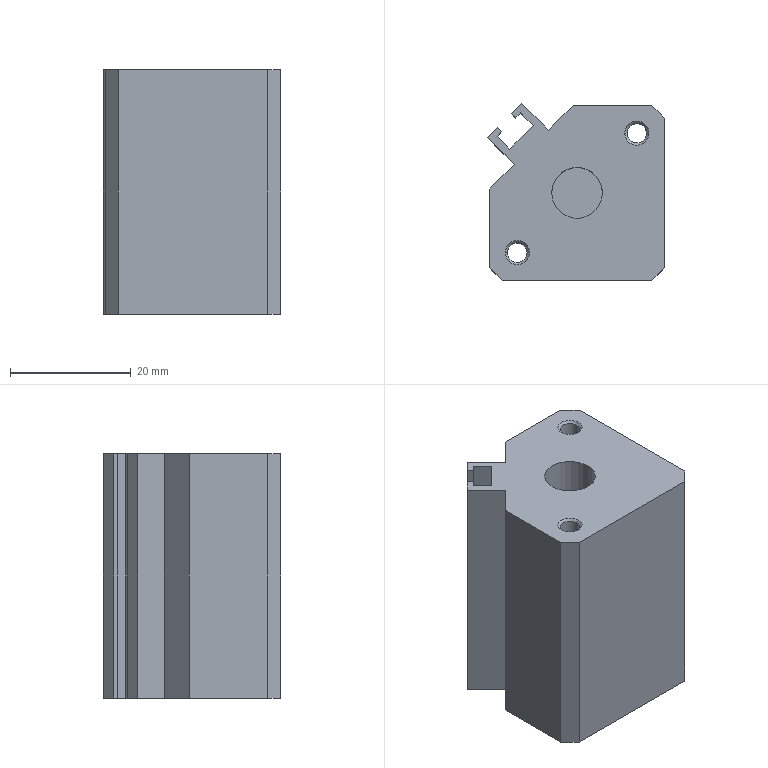Part | SolidWorks | features RevCut 4, Extrusion 1, ICE 1 | 1 solid | 47 faces | box 29.349 x 29.349 x 40.5 mm | volume 29191 mm3 | plane 25 | cone 12 | cylinder 10 | commonest cylinder face diameters 3.24 x4 4.13 x4 8.4 x2
STEP:
#1=CARTESIAN_POINT('',(-4.2,0.,-20.));
#2=VERTEX_POINT('',#1);
#3=CARTESIAN_POINT('',(4.2,0.,-20.));
#4=VERTEX_POINT('',#3);
#5=CARTESIAN_POINT('',(0.,0.,-20.));
#6=DIRECTION('',(0.,0.,1.));
#7=DIRECTION('',(1.,0.,0.));
#8=AXIS2_PLACEMENT_3D('',#5,#6,#7);
#9=CIRCLE('',#8,4.2);
#10=EDGE_CURVE('',#2,#4,#9,.T.);
#11=ORIENTED_EDGE('',*,*,#10,.F.);
#12=CARTESIAN_POINT('',(-4.2,0.,0.));
#13=VERTEX_POINT('',#12);
#14=CARTESIAN_POINT('',(-4.2,0.,-20.));
#15=DIRECTION('',(0.,0.,1.));
#16=VECTOR('',#15,1000.);
#17=LINE('',#14,#16);
#18=EDGE_CURVE('',#2,#13,#17,.T.);
#19=ORIENTED_EDGE('',*,*,#18,.T.);
#20=CARTESIAN_POINT('',(4.2,0.,0.));
#21=VERTEX_POINT('',#20);
#22=CARTESIAN_POINT('',(0.,0.,0.));
#23=DIRECTION('',(0.,0.,1.));
#24=DIRECTION('',(1.,0.,0.));
#25=AXIS2_PLACEMENT_3D('',#22,#23,#24);
#26=CIRCLE('',#25,4.2);
#27=EDGE_CURVE('',#13,#21,#26,.T.);
#28=ORIENTED_EDGE('',*,*,#27,.T.);
#29=CARTESIAN_POINT('',(4.2,0.,-20.));
#30=DIRECTION('',(0.,0.,1.));
#31=VECTOR('',#30,1000.);
#32=LINE('',#29,#31);
#33=EDGE_CURVE('',#4,#21,#32,.T.);
#34=ORIENTED_EDGE('',*,*,#33,.F.);
#35=EDGE_LOOP('',(#11,#19,#28,#34));
#36=FACE_OUTER_BOUND('',#35,.T.);
#37=CARTESIAN_POINT('',(0.,0.,-20.));
#38=DIRECTION('',(0.,0.,1.));
#39=DIRECTION('',(1.,0.,0.));
#40=AXIS2_PLACEMENT_3D('',#37,#38,#39);
#41=CYLINDRICAL_SURFACE('',#40,4.2);
#42=ADVANCED_FACE('',(#36),#41,.F.);
#43=CARTESIAN_POINT('',(-11.519,-9.899,-40.12));
#44=VERTEX_POINT('',#43);
#45=CARTESIAN_POINT('',(-8.279,-9.899,-40.12));
#46=VERTEX_POINT('',#45);
#47=CARTESIAN_POINT('',(-9.899,-9.899,-40.12));
#48=DIRECTION('',(0.,0.,1.));
#49=DIRECTION('',(1.,0.,0.));
#50=AXIS2_PLACEMENT_3D('',#47,#48,#49);
#51=CIRCLE('',#50,1.62);
#52=EDGE_CURVE('',#44,#46,#51,.T.);
#53=ORIENTED_EDGE('',*,*,#52,.F.);
#54=CARTESIAN_POINT('',(-11.519,-9.899,-0.38));
#55=VERTEX_POINT('',#54);
#56=CARTESIAN_POINT('',(-11.519,-9.899,-41.));
#57=DIRECTION('',(0.,0.,1.));
#58=VECTOR('',#57,1000.);
#59=LINE('',#56,#58);
#60=EDGE_CURVE('',#44,#55,#59,.T.);
#61=ORIENTED_EDGE('',*,*,#60,.T.);
#62=CARTESIAN_POINT('',(-8.279,-9.899,-0.38));
#63=VERTEX_POINT('',#62);
#64=CARTESIAN_POINT('',(-9.899,-9.899,-0.38));
#65=DIRECTION('',(0.,0.,1.));
#66=DIRECTION('',(1.,0.,0.));
#67=AXIS2_PLACEMENT_3D('',#64,#65,#66);
#68=CIRCLE('',#67,1.62);
#69=EDGE_CURVE('',#55,#63,#68,.T.);
#70=ORIENTED_EDGE('',*,*,#69,.T.);
#71=CARTESIAN_POINT('',(-8.279,-9.899,-41.));
#72=DIRECTION('',(0.,0.,1.));
#73=VECTOR('',#72,1000.);
#74=LINE('',#71,#73);
#75=EDGE_CURVE('',#46,#63,#74,.T.);
#76=ORIENTED_EDGE('',*,*,#75,.F.);
#77=EDGE_LOOP('',(#53,#61,#70,#76));
#78=FACE_OUTER_BOUND('',#77,.T.);
#79=CARTESIAN_POINT('',(-9.899,-9.899,-41.));
#80=DIRECTION('',(0.,0.,1.));
#81=DIRECTION('',(1.,0.,0.));
#82=AXIS2_PLACEMENT_3D('',#79,#80,#81);
#83=CYLINDRICAL_SURFACE('',#82,1.62);
#84=ADVANCED_FACE('',(#78),#83,.F.);
#85=ORIENTED_EDGE('',*,*,#69,.F.);
#86=CARTESIAN_POINT('',(-11.899,-9.899,0.));
#87=VERTEX_POINT('',#86);
#88=CARTESIAN_POINT('',(-11.519,-9.899,-0.38));
#89=DIRECTION('',(-0.7071,0.,0.7071));
#90=VECTOR('',#89,1000.);
#91=LINE('',#88,#90);
#92=EDGE_CURVE('',#55,#87,#91,.T.);
#93=ORIENTED_EDGE('',*,*,#92,.T.);
#94=CARTESIAN_POINT('',(-7.899,-9.899,0.));
#95=VERTEX_POINT('',#94);
#96=CARTESIAN_POINT('',(-9.899,-9.899,0.));
#97=DIRECTION('',(0.,0.,-1.));
#98=DIRECTION('',(1.,0.,0.));
#99=AXIS2_PLACEMENT_3D('',#96,#97,#98);
#100=CIRCLE('',#99,2.);
#101=EDGE_CURVE('',#95,#87,#100,.T.);
#102=ORIENTED_EDGE('',*,*,#101,.F.);
#103=CARTESIAN_POINT('',(-8.279,-9.899,-0.38));
#104=DIRECTION('',(0.7071,0.,0.7071));
#105=VECTOR('',#104,1000.);
#106=LINE('',#103,#105);
#107=EDGE_CURVE('',#63,#95,#106,.T.);
#108=ORIENTED_EDGE('',*,*,#107,.F.);
#109=EDGE_LOOP('',(#85,#93,#102,#108));
#110=FACE_OUTER_BOUND('',#109,.T.);
#111=CARTESIAN_POINT('',(-9.899,-9.899,-0.38));
#112=DIRECTION('',(0.,0.,1.));
#113=DIRECTION('',(1.,0.,0.));
#114=AXIS2_PLACEMENT_3D('',#111,#112,#113);
#115=CONICAL_SURFACE('',#114,1.62,0.7854);
#116=ADVANCED_FACE('',(#110),#115,.F.);
#117=ORIENTED_EDGE('',*,*,#52,.T.);
#118=CARTESIAN_POINT('',(-7.899,-9.899,-40.5));
#119=VERTEX_POINT('',#118);
#120=CARTESIAN_POINT('',(-7.399,-9.899,-41.));
#121=DIRECTION('',(0.7071,0.,-0.7071));
#122=VECTOR('',#121,1000.);
#123=LINE('',#120,#122);
#124=EDGE_CURVE('',#46,#119,#123,.T.);
#125=ORIENTED_EDGE('',*,*,#124,.T.);
#126=CARTESIAN_POINT('',(-11.899,-9.899,-40.5));
#127=VERTEX_POINT('',#126);
#128=CARTESIAN_POINT('',(-9.899,-9.899,-40.5));
#129=DIRECTION('',(0.,0.,-1.));
#130=DIRECTION('',(1.,0.,0.));
#131=AXIS2_PLACEMENT_3D('',#128,#129,#130);
#132=CIRCLE('',#131,2.);
#133=EDGE_CURVE('',#119,#127,#132,.T.);
#134=ORIENTED_EDGE('',*,*,#133,.T.);
#135=CARTESIAN_POINT('',(-12.399,-9.899,-41.));
#136=DIRECTION('',(-0.7071,0.,-0.7071));
#137=VECTOR('',#136,1000.);
#138=LINE('',#135,#137);
#139=EDGE_CURVE('',#44,#127,#138,.T.);
#140=ORIENTED_EDGE('',*,*,#139,.F.);
#141=EDGE_LOOP('',(#117,#125,#134,#140));
#142=FACE_OUTER_BOUND('',#141,.T.);
#143=CARTESIAN_POINT('',(-9.899,-9.899,-41.));
#144=DIRECTION('',(0.,0.,-1.));
#145=DIRECTION('',(-1.,0.,0.));
#146=AXIS2_PLACEMENT_3D('',#143,#144,#145);
#147=CONICAL_SURFACE('',#146,2.5,0.7854);
#148=ADVANCED_FACE('',(#142),#147,.F.);
#149=CARTESIAN_POINT('',(8.279,9.899,-40.12));
#150=VERTEX_POINT('',#149);
#151=CARTESIAN_POINT('',(11.519,9.899,-40.12));
#152=VERTEX_POINT('',#151);
#153=CARTESIAN_POINT('',(9.899,9.899,-40.12));
#154=DIRECTION('',(0.,0.,1.));
#155=DIRECTION('',(1.,0.,0.));
#156=AXIS2_PLACEMENT_3D('',#153,#154,#155);
#157=CIRCLE('',#156,1.62);
#158=EDGE_CURVE('',#150,#152,#157,.T.);
#159=ORIENTED_EDGE('',*,*,#158,.F.);
#160=CARTESIAN_POINT('',(8.279,9.899,-0.38));
#161=VERTEX_POINT('',#160);
#162=CARTESIAN_POINT('',(8.279,9.899,-41.));
#163=DIRECTION('',(0.,0.,1.));
#164=VECTOR('',#163,1000.);
#165=LINE('',#162,#164);
#166=EDGE_CURVE('',#150,#161,#165,.T.);
#167=ORIENTED_EDGE('',*,*,#166,.T.);
#168=CARTESIAN_POINT('',(11.519,9.899,-0.38));
#169=VERTEX_POINT('',#168);
#170=CARTESIAN_POINT('',(9.899,9.899,-0.38));
#171=DIRECTION('',(0.,0.,1.));
#172=DIRECTION('',(1.,0.,0.));
#173=AXIS2_PLACEMENT_3D('',#170,#171,#172);
#174=CIRCLE('',#173,1.62);
#175=EDGE_CURVE('',#161,#169,#174,.T.);
#176=ORIENTED_EDGE('',*,*,#175,.T.);
#177=CARTESIAN_POINT('',(11.519,9.899,-41.));
#178=DIRECTION('',(0.,0.,1.));
#179=VECTOR('',#178,1000.);
#180=LINE('',#177,#179);
#181=EDGE_CURVE('',#152,#169,#180,.T.);
#182=ORIENTED_EDGE('',*,*,#181,.F.);
#183=EDGE_LOOP('',(#159,#167,#176,#182));
#184=FACE_OUTER_BOUND('',#183,.T.);
#185=CARTESIAN_POINT('',(9.899,9.899,-41.));
#186=DIRECTION('',(0.,0.,1.));
#187=DIRECTION('',(1.,0.,0.));
#188=AXIS2_PLACEMENT_3D('',#185,#186,#187);
#189=CYLINDRICAL_SURFACE('',#188,1.62);
#190=ADVANCED_FACE('',(#184),#189,.F.);
#191=ORIENTED_EDGE('',*,*,#175,.F.);
#192=CARTESIAN_POINT('',(7.899,9.899,0.));
#193=VERTEX_POINT('',#192);
#194=CARTESIAN_POINT('',(8.279,9.899,-0.38));
#195=DIRECTION('',(-0.7071,0.,0.7071));
#196=VECTOR('',#195,1000.);
#197=LINE('',#194,#196);
#198=EDGE_CURVE('',#161,#193,#197,.T.);
#199=ORIENTED_EDGE('',*,*,#198,.T.);
#200=CARTESIAN_POINT('',(11.899,9.899,0.));
#201=VERTEX_POINT('',#200);
#202=CARTESIAN_POINT('',(9.899,9.899,0.));
#203=DIRECTION('',(0.,0.,-1.));
#204=DIRECTION('',(1.,0.,0.));
#205=AXIS2_PLACEMENT_3D('',#202,#203,#204);
#206=CIRCLE('',#205,2.);
#207=EDGE_CURVE('',#201,#193,#206,.T.);
#208=ORIENTED_EDGE('',*,*,#207,.F.);
#209=CARTESIAN_POINT('',(11.519,9.899,-0.38));
#210=DIRECTION('',(0.7071,0.,0.7071));
#211=VECTOR('',#210,1000.);
#212=LINE('',#209,#211);
#213=EDGE_CURVE('',#169,#201,#212,.T.);
#214=ORIENTED_EDGE('',*,*,#213,.F.);
#215=EDGE_LOOP('',(#191,#199,#208,#214));
#216=FACE_OUTER_BOUND('',#215,.T.);
#217=CARTESIAN_POINT('',(9.899,9.899,-0.38));
#218=DIRECTION('',(0.,0.,1.));
#219=DIRECTION('',(1.,0.,0.));
#220=AXIS2_PLACEMENT_3D('',#217,#218,#219);
#221=CONICAL_SURFACE('',#220,1.62,0.7854);
#222=ADVANCED_FACE('',(#216),#221,.F.);
#223=ORIENTED_EDGE('',*,*,#158,.T.);
#224=CARTESIAN_POINT('',(11.899,9.899,-40.5));
#225=VERTEX_POINT('',#224);
#226=CARTESIAN_POINT('',(12.399,9.899,-41.));
#227=DIRECTION('',(0.7071,0.,-0.7071));
#228=VECTOR('',#227,1000.);
#229=LINE('',#226,#228);
#230=EDGE_CURVE('',#152,#225,#229,.T.);
#231=ORIENTED_EDGE('',*,*,#230,.T.);
#232=CARTESIAN_POINT('',(7.899,9.899,-40.5));
#233=VERTEX_POINT('',#232);
#234=CARTESIAN_POINT('',(9.899,9.899,-40.5));
#235=DIRECTION('',(0.,0.,-1.));
#236=DIRECTION('',(1.,0.,0.));
#237=AXIS2_PLACEMENT_3D('',#234,#235,#236);
#238=CIRCLE('',#237,2.);
#239=EDGE_CURVE('',#225,#233,#238,.T.);
#240=ORIENTED_EDGE('',*,*,#239,.T.);
#241=CARTESIAN_POINT('',(7.399,9.899,-41.));
#242=DIRECTION('',(-0.7071,0.,-0.7071));
#243=VECTOR('',#242,1000.);
#244=LINE('',#241,#243);
#245=EDGE_CURVE('',#150,#233,#244,.T.);
#246=ORIENTED_EDGE('',*,*,#245,.F.);
#247=EDGE_LOOP('',(#223,#231,#240,#246));
#248=FACE_OUTER_BOUND('',#247,.T.);
#249=CARTESIAN_POINT('',(9.899,9.899,-41.));
#250=DIRECTION('',(0.,0.,-1.));
#251=DIRECTION('',(-1.,0.,0.));
#252=AXIS2_PLACEMENT_3D('',#249,#250,#251);
#253=CONICAL_SURFACE('',#252,2.5,0.7854);
#254=ADVANCED_FACE('',(#248),#253,.F.);
#255=CARTESIAN_POINT('',(14.065,0.,-37.065));
#256=VERTEX_POINT('',#255);
#257=CARTESIAN_POINT('',(14.065,0.,-32.935));
#258=VERTEX_POINT('',#257);
#259=CARTESIAN_POINT('',(14.065,0.,-35.));
#260=DIRECTION('',(-1.,0.,0.));
#261=DIRECTION('',(0.,0.,1.));
#262=AXIS2_PLACEMENT_3D('',#259,#260,#261);
#263=CIRCLE('',#262,2.065);
#264=EDGE_CURVE('',#256,#258,#263,.T.);
#265=ORIENTED_EDGE('',*,*,#264,.T.);
#266=CARTESIAN_POINT('',(14.5,0.,-32.5));
#267=VERTEX_POINT('',#266);
#268=CARTESIAN_POINT('',(15.,0.,-32.));
#269=DIRECTION('',(0.7071,0.,0.7071));
#270=VECTOR('',#269,1000.);
#271=LINE('',#268,#270);
#272=EDGE_CURVE('',#258,#267,#271,.T.);
#273=ORIENTED_EDGE('',*,*,#272,.T.);
#274=CARTESIAN_POINT('',(14.5,0.,-37.5));
#275=VERTEX_POINT('',#274);
#276=CARTESIAN_POINT('',(14.5,0.,-35.));
#277=DIRECTION('',(-1.,0.,0.));
#278=DIRECTION('',(0.,0.,-1.));
#279=AXIS2_PLACEMENT_3D('',#276,#277,#278);
#280=CIRCLE('',#279,2.5);
#281=EDGE_CURVE('',#275,#267,#280,.T.);
#282=ORIENTED_EDGE('',*,*,#281,.F.);
#283=CARTESIAN_POINT('',(15.,0.,-38.));
#284=DIRECTION('',(0.7071,0.,-0.7071));
#285=VECTOR('',#284,1000.);
#286=LINE('',#283,#285);
#287=EDGE_CURVE('',#256,#275,#286,.T.);
#288=ORIENTED_EDGE('',*,*,#287,.F.);
#289=EDGE_LOOP('',(#265,#273,#282,#288));
#290=FACE_OUTER_BOUND('',#289,.T.);
#291=CARTESIAN_POINT('',(15.,0.,-35.));
#292=DIRECTION('',(1.,0.,0.));
#293=DIRECTION('',(0.,0.,-1.));
#294=AXIS2_PLACEMENT_3D('',#291,#292,#293);
#295=CONICAL_SURFACE('',#294,3.,0.7854);
#296=ADVANCED_FACE('',(#290),#295,.F.);
#297=ORIENTED_EDGE('',*,*,#264,.F.);
#298=CARTESIAN_POINT('',(8.5,0.,-37.065));
#299=VERTEX_POINT('',#298);
#300=CARTESIAN_POINT('',(15.,0.,-37.065));
#301=DIRECTION('',(-1.,0.,0.));
#302=VECTOR('',#301,1000.);
#303=LINE('',#300,#302);
#304=EDGE_CURVE('',#256,#299,#303,.T.);
#305=ORIENTED_EDGE('',*,*,#304,.T.);
#306=CARTESIAN_POINT('',(8.5,0.,-32.935));
#307=VERTEX_POINT('',#306);
#308=CARTESIAN_POINT('',(8.5,0.,-35.));
#309=DIRECTION('',(-1.,0.,0.));
#310=DIRECTION('',(0.,0.,1.));
#311=AXIS2_PLACEMENT_3D('',#308,#309,#310);
#312=CIRCLE('',#311,2.065);
#313=EDGE_CURVE('',#299,#307,#312,.T.);
#314=ORIENTED_EDGE('',*,*,#313,.T.);
#315=CARTESIAN_POINT('',(15.,0.,-32.935));
#316=DIRECTION('',(-1.,0.,0.));
#317=VECTOR('',#316,1000.);
#318=LINE('',#315,#317);
#319=EDGE_CURVE('',#258,#307,#318,.T.);
#320=ORIENTED_EDGE('',*,*,#319,.F.);
#321=EDGE_LOOP('',(#297,#305,#314,#320));
#322=FACE_OUTER_BOUND('',#321,.T.);
#323=CARTESIAN_POINT('',(15.,0.,-35.));
#324=DIRECTION('',(-1.,0.,0.));
#325=DIRECTION('',(0.,0.,1.));
#326=AXIS2_PLACEMENT_3D('',#323,#324,#325);
#327=CYLINDRICAL_SURFACE('',#326,2.065);
#328=ADVANCED_FACE('',(#322),#327,.F.);
#329=CARTESIAN_POINT('',(14.065,0.,-12.065));
#330=VERTEX_POINT('',#329);
#331=CARTESIAN_POINT('',(14.065,0.,-7.935));
#332=VERTEX_POINT('',#331);
#333=CARTESIAN_POINT('',(14.065,0.,-10.));
#334=DIRECTION('',(-1.,0.,0.));
#335=DIRECTION('',(0.,0.,1.));
#336=AXIS2_PLACEMENT_3D('',#333,#334,#335);
#337=CIRCLE('',#336,2.065);
#338=EDGE_CURVE('',#330,#332,#337,.T.);
#339=ORIENTED_EDGE('',*,*,#338,.T.);
#340=CARTESIAN_POINT('',(14.5,0.,-7.5));
#341=VERTEX_POINT('',#340);
#342=CARTESIAN_POINT('',(15.,0.,-7.));
#343=DIRECTION('',(0.7071,0.,0.7071));
#344=VECTOR('',#343,1000.);
#345=LINE('',#342,#344);
#346=EDGE_CURVE('',#332,#341,#345,.T.);
#347=ORIENTED_EDGE('',*,*,#346,.T.);
#348=CARTESIAN_POINT('',(14.5,0.,-12.5));
#349=VERTEX_POINT('',#348);
#350=CARTESIAN_POINT('',(14.5,0.,-10.));
#351=DIRECTION('',(-1.,0.,0.));
#352=DIRECTION('',(0.,0.,-1.));
#353=AXIS2_PLACEMENT_3D('',#350,#351,#352);
#354=CIRCLE('',#353,2.5);
#355=EDGE_CURVE('',#349,#341,#354,.T.);
#356=ORIENTED_EDGE('',*,*,#355,.F.);
#357=CARTESIAN_POINT('',(15.,0.,-13.));
#358=DIRECTION('',(0.7071,0.,-0.7071));
#359=VECTOR('',#358,1000.);
#360=LINE('',#357,#359);
#361=EDGE_CURVE('',#330,#349,#360,.T.);
#362=ORIENTED_EDGE('',*,*,#361,.F.);
#363=EDGE_LOOP('',(#339,#347,#356,#362));
#364=FACE_OUTER_BOUND('',#363,.T.);
#365=CARTESIAN_POINT('',(15.,0.,-10.));
#366=DIRECTION('',(1.,0.,0.));
#367=DIRECTION('',(0.,0.,-1.));
#368=AXIS2_PLACEMENT_3D('',#365,#366,#367);
#369=CONICAL_SURFACE('',#368,3.,0.7854);
#370=ADVANCED_FACE('',(#364),#369,.F.);
#371=ORIENTED_EDGE('',*,*,#338,.F.);
#372=CARTESIAN_POINT('',(8.5,0.,-12.065));
#373=VERTEX_POINT('',#372);
#374=CARTESIAN_POINT('',(15.,0.,-12.065));
#375=DIRECTION('',(-1.,0.,0.));
#376=VECTOR('',#375,1000.);
#377=LINE('',#374,#376);
#378=EDGE_CURVE('',#330,#373,#377,.T.);
#379=ORIENTED_EDGE('',*,*,#378,.T.);
#380=CARTESIAN_POINT('',(8.5,0.,-7.935));
#381=VERTEX_POINT('',#380);
#382=CARTESIAN_POINT('',(8.5,0.,-10.));
#383=DIRECTION('',(-1.,0.,0.));
#384=DIRECTION('',(0.,0.,1.));
#385=AXIS2_PLACEMENT_3D('',#382,#383,#384);
#386=CIRCLE('',#385,2.065);
#387=EDGE_CURVE('',#373,#381,#386,.T.);
#388=ORIENTED_EDGE('',*,*,#387,.T.);
#389=CARTESIAN_POINT('',(15.,0.,-7.935));
#390=DIRECTION('',(-1.,0.,0.));
#391=VECTOR('',#390,1000.);
#392=LINE('',#389,#391);
#393=EDGE_CURVE('',#332,#381,#392,.T.);
#394=ORIENTED_EDGE('',*,*,#393,.F.);
#395=EDGE_LOOP('',(#371,#379,#388,#394));
#396=FACE_OUTER_BOUND('',#395,.T.);
#397=CARTESIAN_POINT('',(15.,0.,-10.));
#398=DIRECTION('',(-1.,0.,0.));
#399=DIRECTION('',(0.,0.,1.));
#400=AXIS2_PLACEMENT_3D('',#397,#398,#399);
#401=CYLINDRICAL_SURFACE('',#400,2.065);
#402=ADVANCED_FACE('',(#396),#401,.F.);
#403=CARTESIAN_POINT('',(9.899,9.899,-40.5));
#404=DIRECTION('',(0.,0.,-1.));
#405=DIRECTION('',(1.,0.,0.));
#406=AXIS2_PLACEMENT_3D('',#403,#404,#405);
#407=CIRCLE('',#406,2.);
#408=EDGE_CURVE('',#233,#225,#407,.T.);
#409=ORIENTED_EDGE('',*,*,#408,.F.);
#410=ORIENTED_EDGE('',*,*,#239,.F.);
#411=EDGE_LOOP('',(#409,#410));
#412=FACE_BOUND('',#411,.T.);
#413=CARTESIAN_POINT('',(-13.152,10.889,-40.5));
#414=VERTEX_POINT('',#413);
#415=CARTESIAN_POINT('',(-14.849,9.192,-40.5));
#416=VERTEX_POINT('',#415);
#417=CARTESIAN_POINT('',(-13.152,10.889,-40.5));
#418=DIRECTION('',(-0.7071,-0.7071,0.));
#419=VECTOR('',#418,1000.);
#420=LINE('',#417,#419);
#421=EDGE_CURVE('',#414,#416,#420,.T.);
#422=ORIENTED_EDGE('',*,*,#421,.F.);
#423=CARTESIAN_POINT('',(-12.445,10.182,-40.5));
#424=VERTEX_POINT('',#423);
#425=CARTESIAN_POINT('',(-12.445,10.182,-40.5));
#426=DIRECTION('',(-0.7071,0.7071,0.));
#427=VECTOR('',#426,1000.);
#428=LINE('',#425,#427);
#429=EDGE_CURVE('',#424,#414,#428,.T.);
#430=ORIENTED_EDGE('',*,*,#429,.F.);
#431=CARTESIAN_POINT('',(-13.258,9.369,-40.5));
#432=VERTEX_POINT('',#431);
#433=CARTESIAN_POINT('',(-13.258,9.369,-40.5));
#434=DIRECTION('',(0.7071,0.7071,0.));
#435=VECTOR('',#434,1000.);
#436=LINE('',#433,#435);
#437=EDGE_CURVE('',#432,#424,#436,.T.);
#438=ORIENTED_EDGE('',*,*,#437,.F.);
#439=CARTESIAN_POINT('',(-11.137,7.248,-40.5));
#440=VERTEX_POINT('',#439);
#441=CARTESIAN_POINT('',(-11.137,7.248,-40.5));
#442=DIRECTION('',(-0.7071,0.7071,0.));
#443=VECTOR('',#442,1000.);
#444=LINE('',#441,#443);
#445=EDGE_CURVE('',#440,#432,#444,.T.);
#446=ORIENTED_EDGE('',*,*,#445,.F.);
#447=CARTESIAN_POINT('',(-7.248,11.137,-40.5));
#448=VERTEX_POINT('',#447);
#449=CARTESIAN_POINT('',(-7.248,11.137,-40.5));
#450=DIRECTION('',(-0.7071,-0.7071,0.));
#451=VECTOR('',#450,1000.);
#452=LINE('',#449,#451);
#453=EDGE_CURVE('',#448,#440,#452,.T.);
#454=ORIENTED_EDGE('',*,*,#453,.F.);
#455=CARTESIAN_POINT('',(-9.369,13.258,-40.5));
#456=VERTEX_POINT('',#455);
#457=CARTESIAN_POINT('',(-9.369,13.258,-40.5));
#458=DIRECTION('',(0.7071,-0.7071,0.));
#459=VECTOR('',#458,1000.);
#460=LINE('',#457,#459);
#461=EDGE_CURVE('',#456,#448,#460,.T.);
#462=ORIENTED_EDGE('',*,*,#461,.F.);
#463=CARTESIAN_POINT('',(-10.182,12.445,-40.5));
#464=VERTEX_POINT('',#463);
#465=CARTESIAN_POINT('',(-10.182,12.445,-40.5));
#466=DIRECTION('',(0.7071,0.7071,0.));
#467=VECTOR('',#466,1000.);
#468=LINE('',#465,#467);
#469=EDGE_CURVE('',#464,#456,#468,.T.);
#470=ORIENTED_EDGE('',*,*,#469,.F.);
#471=CARTESIAN_POINT('',(-10.889,13.152,-40.5));
#472=VERTEX_POINT('',#471);
#473=CARTESIAN_POINT('',(-10.889,13.152,-40.5));
#474=DIRECTION('',(0.7071,-0.7071,0.));
#475=VECTOR('',#474,1000.);
#476=LINE('',#473,#475);
#477=EDGE_CURVE('',#472,#464,#476,.T.);
#478=ORIENTED_EDGE('',*,*,#477,.F.);
#479=CARTESIAN_POINT('',(-9.192,14.849,-40.5));
#480=VERTEX_POINT('',#479);
#481=CARTESIAN_POINT('',(-9.192,14.849,-40.5));
#482=DIRECTION('',(-0.7071,-0.7071,0.));
#483=VECTOR('',#482,1000.);
#484=LINE('',#481,#483);
#485=EDGE_CURVE('',#480,#472,#484,.T.);
#486=ORIENTED_EDGE('',*,*,#485,.F.);
#487=CARTESIAN_POINT('',(-4.738,10.394,-40.5));
#488=VERTEX_POINT('',#487);
#489=CARTESIAN_POINT('',(-4.738,10.394,-40.5));
#490=DIRECTION('',(-0.7071,0.7071,0.));
#491=VECTOR('',#490,1000.);
#492=LINE('',#489,#491);
#493=EDGE_CURVE('',#488,#480,#492,.T.);
#494=ORIENTED_EDGE('',*,*,#493,.F.);
#495=CARTESIAN_POINT('',(-0.6321,14.5,-40.5));
#496=VERTEX_POINT('',#495);
#497=CARTESIAN_POINT('',(-0.6321,14.5,-40.5));
#498=DIRECTION('',(-0.7071,-0.7071,0.));
#499=VECTOR('',#498,1000.);
#500=LINE('',#497,#499);
#501=EDGE_CURVE('',#496,#488,#500,.T.);
#502=ORIENTED_EDGE('',*,*,#501,.F.);
#503=CARTESIAN_POINT('',(12.37,14.5,-40.5));
#504=VERTEX_POINT('',#503);
#505=CARTESIAN_POINT('',(12.37,14.5,-40.5));
#506=DIRECTION('',(-1.,0.,0.));
#507=VECTOR('',#506,1000.);
#508=LINE('',#505,#507);
#509=EDGE_CURVE('',#504,#496,#508,.T.);
#510=ORIENTED_EDGE('',*,*,#509,.F.);
#511=CARTESIAN_POINT('',(14.5,12.37,-40.5));
#512=VERTEX_POINT('',#511);
#513=CARTESIAN_POINT('',(14.5,12.37,-40.5));
#514=DIRECTION('',(-0.7071,0.7071,0.));
#515=VECTOR('',#514,1000.);
#516=LINE('',#513,#515);
#517=EDGE_CURVE('',#512,#504,#516,.T.);
#518=ORIENTED_EDGE('',*,*,#517,.F.);
#519=CARTESIAN_POINT('',(14.5,-12.37,-40.5));
#520=VERTEX_POINT('',#519);
#521=CARTESIAN_POINT('',(14.5,-12.37,-40.5));
#522=DIRECTION('',(0.,1.,0.));
#523=VECTOR('',#522,1000.);
#524=LINE('',#521,#523);
#525=EDGE_CURVE('',#520,#512,#524,.T.);
#526=ORIENTED_EDGE('',*,*,#525,.F.);
#527=CARTESIAN_POINT('',(12.37,-14.5,-40.5));
#528=VERTEX_POINT('',#527);
#529=CARTESIAN_POINT('',(12.37,-14.5,-40.5));
#530=DIRECTION('',(0.7071,0.7071,0.));
#531=VECTOR('',#530,1000.);
#532=LINE('',#529,#531);
#533=EDGE_CURVE('',#528,#520,#532,.T.);
#534=ORIENTED_EDGE('',*,*,#533,.F.);
#535=CARTESIAN_POINT('',(-12.37,-14.5,-40.5));
#536=VERTEX_POINT('',#535);
#537=CARTESIAN_POINT('',(-12.37,-14.5,-40.5));
#538=DIRECTION('',(1.,0.,0.));
#539=VECTOR('',#538,1000.);
#540=LINE('',#537,#539);
#541=EDGE_CURVE('',#536,#528,#540,.T.);
#542=ORIENTED_EDGE('',*,*,#541,.F.);
#543=CARTESIAN_POINT('',(-14.5,-12.37,-40.5));
#544=VERTEX_POINT('',#543);
#545=CARTESIAN_POINT('',(-14.5,-12.37,-40.5));
#546=DIRECTION('',(0.7071,-0.7071,0.));
#547=VECTOR('',#546,1000.);
#548=LINE('',#545,#547);
#549=EDGE_CURVE('',#544,#536,#548,.T.);
#550=ORIENTED_EDGE('',*,*,#549,.F.);
#551=CARTESIAN_POINT('',(-14.5,0.6321,-40.5));
#552=VERTEX_POINT('',#551);
#553=CARTESIAN_POINT('',(-14.5,0.6321,-40.5));
#554=DIRECTION('',(0.,-1.,0.));
#555=VECTOR('',#554,1000.);
#556=LINE('',#553,#555);
#557=EDGE_CURVE('',#552,#544,#556,.T.);
#558=ORIENTED_EDGE('',*,*,#557,.F.);
#559=CARTESIAN_POINT('',(-10.394,4.738,-40.5));
#560=VERTEX_POINT('',#559);
#561=CARTESIAN_POINT('',(-10.394,4.738,-40.5));
#562=DIRECTION('',(-0.7071,-0.7071,0.));
#563=VECTOR('',#562,1000.);
#564=LINE('',#561,#563);
#565=EDGE_CURVE('',#560,#552,#564,.T.);
#566=ORIENTED_EDGE('',*,*,#565,.F.);
#567=CARTESIAN_POINT('',(-14.849,9.192,-40.5));
#568=DIRECTION('',(0.7071,-0.7071,0.));
#569=VECTOR('',#568,1000.);
#570=LINE('',#567,#569);
#571=EDGE_CURVE('',#416,#560,#570,.T.);
#572=ORIENTED_EDGE('',*,*,#571,.F.);
#573=EDGE_LOOP('',(#422,#430,#438,#446,#454,#462,#470,#478,#486,#494,#502,#510,#518,#526,#534,#542,#550,#558,#566,#572));
#574=FACE_OUTER_BOUND('',#573,.T.);
#575=CARTESIAN_POINT('',(-9.899,-9.899,-40.5));
#576=DIRECTION('',(0.,0.,-1.));
#577=DIRECTION('',(1.,0.,0.));
#578=AXIS2_PLACEMENT_3D('',#575,#576,#577);
#579=CIRCLE('',#578,2.);
#580=EDGE_CURVE('',#127,#119,#579,.T.);
#581=ORIENTED_EDGE('',*,*,#580,.F.);
#582=ORIENTED_EDGE('',*,*,#133,.F.);
#583=EDGE_LOOP('',(#581,#582));
#584=FACE_BOUND('',#583,.T.);
#585=CARTESIAN_POINT('',(0.,0.,-40.5));
#586=DIRECTION('',(0.,0.,1.));
#587=DIRECTION('',(1.,0.,0.));
#588=AXIS2_PLACEMENT_3D('',#585,#586,#587);
#589=PLANE('',#588);
#590=ADVANCED_FACE('',(#412,#574,#584),#589,.F.);
#591=CARTESIAN_POINT('',(0.,0.,0.));
#592=DIRECTION('',(0.,0.,1.));
#593=DIRECTION('',(1.,0.,0.));
#594=AXIS2_PLACEMENT_3D('',#591,#592,#593);
#595=CIRCLE('',#594,4.2);
#596=EDGE_CURVE('',#21,#13,#595,.T.);
#597=ORIENTED_EDGE('',*,*,#596,.F.);
#598=ORIENTED_EDGE('',*,*,#27,.F.);
#599=EDGE_LOOP('',(#597,#598));
#600=FACE_BOUND('',#599,.T.);
#601=ORIENTED_EDGE('',*,*,#207,.T.);
#602=CARTESIAN_POINT('',(9.899,9.899,0.));
#603=DIRECTION('',(0.,0.,-1.));
#604=DIRECTION('',(1.,0.,0.));
#605=AXIS2_PLACEMENT_3D('',#602,#603,#604);
#606=CIRCLE('',#605,2.);
#607=EDGE_CURVE('',#193,#201,#606,.T.);
#608=ORIENTED_EDGE('',*,*,#607,.T.);
#609=EDGE_LOOP('',(#601,#608));
#610=FACE_BOUND('',#609,.T.);
#611=CARTESIAN_POINT('',(-13.152,10.889,0.));
#612=VERTEX_POINT('',#611);
#613=CARTESIAN_POINT('',(-14.849,9.192,0.));
#614=VERTEX_POINT('',#613);
#615=CARTESIAN_POINT('',(-13.152,10.889,0.));
#616=DIRECTION('',(-0.7071,-0.7071,0.));
#617=VECTOR('',#616,1000.);
#618=LINE('',#615,#617);
#619=EDGE_CURVE('',#612,#614,#618,.T.);
#620=ORIENTED_EDGE('',*,*,#619,.T.);
#621=CARTESIAN_POINT('',(-10.394,4.738,0.));
#622=VERTEX_POINT('',#621);
#623=CARTESIAN_POINT('',(-14.849,9.192,0.));
#624=DIRECTION('',(0.7071,-0.7071,0.));
#625=VECTOR('',#624,1000.);
#626=LINE('',#623,#625);
#627=EDGE_CURVE('',#614,#622,#626,.T.);
#628=ORIENTED_EDGE('',*,*,#627,.T.);
#629=CARTESIAN_POINT('',(-14.5,0.6321,0.));
#630=VERTEX_POINT('',#629);
#631=CARTESIAN_POINT('',(-10.394,4.738,0.));
#632=DIRECTION('',(-0.7071,-0.7071,0.));
#633=VECTOR('',#632,1000.);
#634=LINE('',#631,#633);
#635=EDGE_CURVE('',#622,#630,#634,.T.);
#636=ORIENTED_EDGE('',*,*,#635,.T.);
#637=CARTESIAN_POINT('',(-14.5,-12.37,0.));
#638=VERTEX_POINT('',#637);
#639=CARTESIAN_POINT('',(-14.5,0.6321,0.));
#640=DIRECTION('',(0.,-1.,0.));
#641=VECTOR('',#640,1000.);
#642=LINE('',#639,#641);
#643=EDGE_CURVE('',#630,#638,#642,.T.);
#644=ORIENTED_EDGE('',*,*,#643,.T.);
#645=CARTESIAN_POINT('',(-12.37,-14.5,0.));
#646=VERTEX_POINT('',#645);
#647=CARTESIAN_POINT('',(-14.5,-12.37,0.));
#648=DIRECTION('',(0.7071,-0.7071,0.));
#649=VECTOR('',#648,1000.);
#650=LINE('',#647,#649);
#651=EDGE_CURVE('',#638,#646,#650,.T.);
#652=ORIENTED_EDGE('',*,*,#651,.T.);
#653=CARTESIAN_POINT('',(12.37,-14.5,0.));
#654=VERTEX_POINT('',#653);
#655=CARTESIAN_POINT('',(-12.37,-14.5,0.));
#656=DIRECTION('',(1.,0.,0.));
#657=VECTOR('',#656,1000.);
#658=LINE('',#655,#657);
#659=EDGE_CURVE('',#646,#654,#658,.T.);
#660=ORIENTED_EDGE('',*,*,#659,.T.);
#661=CARTESIAN_POINT('',(14.5,-12.37,0.));
#662=VERTEX_POINT('',#661);
#663=CARTESIAN_POINT('',(12.37,-14.5,0.));
#664=DIRECTION('',(0.7071,0.7071,0.));
#665=VECTOR('',#664,1000.);
#666=LINE('',#663,#665);
#667=EDGE_CURVE('',#654,#662,#666,.T.);
#668=ORIENTED_EDGE('',*,*,#667,.T.);
#669=CARTESIAN_POINT('',(14.5,12.37,0.));
#670=VERTEX_POINT('',#669);
#671=CARTESIAN_POINT('',(14.5,-12.37,0.));
#672=DIRECTION('',(0.,1.,0.));
#673=VECTOR('',#672,1000.);
#674=LINE('',#671,#673);
#675=EDGE_CURVE('',#662,#670,#674,.T.);
#676=ORIENTED_EDGE('',*,*,#675,.T.);
#677=CARTESIAN_POINT('',(12.37,14.5,0.));
#678=VERTEX_POINT('',#677);
#679=CARTESIAN_POINT('',(14.5,12.37,0.));
#680=DIRECTION('',(-0.7071,0.7071,0.));
#681=VECTOR('',#680,1000.);
#682=LINE('',#679,#681);
#683=EDGE_CURVE('',#670,#678,#682,.T.);
#684=ORIENTED_EDGE('',*,*,#683,.T.);
#685=CARTESIAN_POINT('',(-0.6321,14.5,0.));
#686=VERTEX_POINT('',#685);
#687=CARTESIAN_POINT('',(12.37,14.5,0.));
#688=DIRECTION('',(-1.,0.,0.));
#689=VECTOR('',#688,1000.);
#690=LINE('',#687,#689);
#691=EDGE_CURVE('',#678,#686,#690,.T.);
#692=ORIENTED_EDGE('',*,*,#691,.T.);
#693=CARTESIAN_POINT('',(-4.738,10.394,0.));
#694=VERTEX_POINT('',#693);
#695=CARTESIAN_POINT('',(-0.6321,14.5,0.));
#696=DIRECTION('',(-0.7071,-0.7071,0.));
#697=VECTOR('',#696,1000.);
#698=LINE('',#695,#697);
#699=EDGE_CURVE('',#686,#694,#698,.T.);
#700=ORIENTED_EDGE('',*,*,#699,.T.);
#701=CARTESIAN_POINT('',(-9.192,14.849,0.));
#702=VERTEX_POINT('',#701);
#703=CARTESIAN_POINT('',(-4.738,10.394,0.));
#704=DIRECTION('',(-0.7071,0.7071,0.));
#705=VECTOR('',#704,1000.);
#706=LINE('',#703,#705);
#707=EDGE_CURVE('',#694,#702,#706,.T.);
#708=ORIENTED_EDGE('',*,*,#707,.T.);
#709=CARTESIAN_POINT('',(-10.889,13.152,0.));
#710=VERTEX_POINT('',#709);
#711=CARTESIAN_POINT('',(-9.192,14.849,0.));
#712=DIRECTION('',(-0.7071,-0.7071,0.));
#713=VECTOR('',#712,1000.);
#714=LINE('',#711,#713);
#715=EDGE_CURVE('',#702,#710,#714,.T.);
#716=ORIENTED_EDGE('',*,*,#715,.T.);
#717=CARTESIAN_POINT('',(-10.182,12.445,0.));
#718=VERTEX_POINT('',#717);
#719=CARTESIAN_POINT('',(-10.889,13.152,0.));
#720=DIRECTION('',(0.7071,-0.7071,0.));
#721=VECTOR('',#720,1000.);
#722=LINE('',#719,#721);
#723=EDGE_CURVE('',#710,#718,#722,.T.);
#724=ORIENTED_EDGE('',*,*,#723,.T.);
#725=CARTESIAN_POINT('',(-9.369,13.258,0.));
#726=VERTEX_POINT('',#725);
#727=CARTESIAN_POINT('',(-10.182,12.445,0.));
#728=DIRECTION('',(0.7071,0.7071,0.));
#729=VECTOR('',#728,1000.);
#730=LINE('',#727,#729);
#731=EDGE_CURVE('',#718,#726,#730,.T.);
#732=ORIENTED_EDGE('',*,*,#731,.T.);
#733=CARTESIAN_POINT('',(-7.248,11.137,0.));
#734=VERTEX_POINT('',#733);
#735=CARTESIAN_POINT('',(-9.369,13.258,0.));
#736=DIRECTION('',(0.7071,-0.7071,0.));
#737=VECTOR('',#736,1000.);
#738=LINE('',#735,#737);
#739=EDGE_CURVE('',#726,#734,#738,.T.);
#740=ORIENTED_EDGE('',*,*,#739,.T.);
#741=CARTESIAN_POINT('',(-11.137,7.248,0.));
#742=VERTEX_POINT('',#741);
#743=CARTESIAN_POINT('',(-7.248,11.137,0.));
#744=DIRECTION('',(-0.7071,-0.7071,0.));
#745=VECTOR('',#744,1000.);
#746=LINE('',#743,#745);
#747=EDGE_CURVE('',#734,#742,#746,.T.);
#748=ORIENTED_EDGE('',*,*,#747,.T.);
#749=CARTESIAN_POINT('',(-13.258,9.369,0.));
#750=VERTEX_POINT('',#749);
#751=CARTESIAN_POINT('',(-11.137,7.248,0.));
#752=DIRECTION('',(-0.7071,0.7071,0.));
#753=VECTOR('',#752,1000.);
#754=LINE('',#751,#753);
#755=EDGE_CURVE('',#742,#750,#754,.T.);
#756=ORIENTED_EDGE('',*,*,#755,.T.);
#757=CARTESIAN_POINT('',(-12.445,10.182,0.));
#758=VERTEX_POINT('',#757);
#759=CARTESIAN_POINT('',(-13.258,9.369,0.));
#760=DIRECTION('',(0.7071,0.7071,0.));
#761=VECTOR('',#760,1000.);
#762=LINE('',#759,#761);
#763=EDGE_CURVE('',#750,#758,#762,.T.);
#764=ORIENTED_EDGE('',*,*,#763,.T.);
#765=CARTESIAN_POINT('',(-12.445,10.182,0.));
#766=DIRECTION('',(-0.7071,0.7071,0.));
#767=VECTOR('',#766,1000.);
#768=LINE('',#765,#767);
#769=EDGE_CURVE('',#758,#612,#768,.T.);
#770=ORIENTED_EDGE('',*,*,#769,.T.);
#771=EDGE_LOOP('',(#620,#628,#636,#644,#652,#660,#668,#676,#684,#692,#700,#708,#716,#724,#732,#740,#748,#756,#764,#770));
#772=FACE_OUTER_BOUND('',#771,.T.);
#773=ORIENTED_EDGE('',*,*,#101,.T.);
#774=CARTESIAN_POINT('',(-9.899,-9.899,0.));
#775=DIRECTION('',(0.,0.,-1.));
#776=DIRECTION('',(1.,0.,0.));
#777=AXIS2_PLACEMENT_3D('',#774,#775,#776);
#778=CIRCLE('',#777,2.);
#779=EDGE_CURVE('',#87,#95,#778,.T.);
#780=ORIENTED_EDGE('',*,*,#779,.T.);
#781=EDGE_LOOP('',(#773,#780));
#782=FACE_BOUND('',#781,.T.);
#783=CARTESIAN_POINT('',(0.,0.,0.));
#784=DIRECTION('',(0.,0.,1.));
#785=DIRECTION('',(1.,0.,0.));
#786=AXIS2_PLACEMENT_3D('',#783,#784,#785);
#787=PLANE('',#786);
#788=ADVANCED_FACE('',(#600,#610,#772,#782),#787,.T.);
#789=ORIENTED_EDGE('',*,*,#355,.T.);
#790=CARTESIAN_POINT('',(14.5,0.,-10.));
#791=DIRECTION('',(-1.,0.,0.));
#792=DIRECTION('',(0.,0.,-1.));
#793=AXIS2_PLACEMENT_3D('',#790,#791,#792);
#794=CIRCLE('',#793,2.5);
#795=EDGE_CURVE('',#341,#349,#794,.T.);
#796=ORIENTED_EDGE('',*,*,#795,.T.);
#797=EDGE_LOOP('',(#789,#796));
#798=FACE_BOUND('',#797,.T.);
#799=ORIENTED_EDGE('',*,*,#675,.F.);
#800=CARTESIAN_POINT('',(14.5,-12.37,-40.5));
#801=DIRECTION('',(0.,0.,1.));
#802=VECTOR('',#801,1000.);
#803=LINE('',#800,#802);
#804=EDGE_CURVE('',#520,#662,#803,.T.);
#805=ORIENTED_EDGE('',*,*,#804,.F.);
#806=ORIENTED_EDGE('',*,*,#525,.T.);
#807=CARTESIAN_POINT('',(14.5,12.37,-40.5));
#808=DIRECTION('',(0.,0.,1.));
#809=VECTOR('',#808,1000.);
#810=LINE('',#807,#809);
#811=EDGE_CURVE('',#512,#670,#810,.T.);
#812=ORIENTED_EDGE('',*,*,#811,.T.);
#813=EDGE_LOOP('',(#799,#805,#806,#812));
#814=FACE_OUTER_BOUND('',#813,.T.);
#815=ORIENTED_EDGE('',*,*,#281,.T.);
#816=CARTESIAN_POINT('',(14.5,0.,-35.));
#817=DIRECTION('',(-1.,0.,0.));
#818=DIRECTION('',(0.,0.,-1.));
#819=AXIS2_PLACEMENT_3D('',#816,#817,#818);
#820=CIRCLE('',#819,2.5);
#821=EDGE_CURVE('',#267,#275,#820,.T.);
#822=ORIENTED_EDGE('',*,*,#821,.T.);
#823=EDGE_LOOP('',(#815,#822));
#824=FACE_BOUND('',#823,.T.);
#825=CARTESIAN_POINT('',(14.5,-12.37,-40.5));
#826=DIRECTION('',(1.,0.,0.));
#827=DIRECTION('',(0.,0.,-1.));
#828=AXIS2_PLACEMENT_3D('',#825,#826,#827);
#829=PLANE('',#828);
#830=ADVANCED_FACE('',(#798,#814,#824),#829,.T.);
#831=ORIENTED_EDGE('',*,*,#619,.F.);
#832=CARTESIAN_POINT('',(-13.152,10.889,-40.5));
#833=DIRECTION('',(0.,0.,1.));
#834=VECTOR('',#833,1000.);
#835=LINE('',#832,#834);
#836=EDGE_CURVE('',#414,#612,#835,.T.);
#837=ORIENTED_EDGE('',*,*,#836,.F.);
#838=ORIENTED_EDGE('',*,*,#421,.T.);
#839=CARTESIAN_POINT('',(-14.849,9.192,-40.5));
#840=DIRECTION('',(0.,0.,1.));
#841=VECTOR('',#840,1000.);
#842=LINE('',#839,#841);
#843=EDGE_CURVE('',#416,#614,#842,.T.);
#844=ORIENTED_EDGE('',*,*,#843,.T.);
#845=EDGE_LOOP('',(#831,#837,#838,#844));
#846=FACE_OUTER_BOUND('',#845,.T.);
#847=CARTESIAN_POINT('',(-13.152,10.889,-40.5));
#848=DIRECTION('',(-0.7071,0.7071,0.));
#849=DIRECTION('',(-0.7071,-0.7071,0.));
#850=AXIS2_PLACEMENT_3D('',#847,#848,#849);
#851=PLANE('',#850);
#852=ADVANCED_FACE('',(#846),#851,.T.);
#853=ORIENTED_EDGE('',*,*,#769,.F.);
#854=CARTESIAN_POINT('',(-12.445,10.182,-40.5));
#855=DIRECTION('',(0.,0.,1.));
#856=VECTOR('',#855,1000.);
#857=LINE('',#854,#856);
#858=EDGE_CURVE('',#424,#758,#857,.T.);
#859=ORIENTED_EDGE('',*,*,#858,.F.);
#860=ORIENTED_EDGE('',*,*,#429,.T.);
#861=ORIENTED_EDGE('',*,*,#836,.T.);
#862=EDGE_LOOP('',(#853,#859,#860,#861));
#863=FACE_OUTER_BOUND('',#862,.T.);
#864=CARTESIAN_POINT('',(-12.445,10.182,-40.5));
#865=DIRECTION('',(0.7071,0.7071,0.));
#866=DIRECTION('',(-0.7071,0.7071,0.));
#867=AXIS2_PLACEMENT_3D('',#864,#865,#866);
#868=PLANE('',#867);
#869=ADVANCED_FACE('',(#863),#868,.T.);
#870=ORIENTED_EDGE('',*,*,#763,.F.);
#871=CARTESIAN_POINT('',(-13.258,9.369,-40.5));
#872=DIRECTION('',(0.,0.,1.));
#873=VECTOR('',#872,1000.);
#874=LINE('',#871,#873);
#875=EDGE_CURVE('',#432,#750,#874,.T.);
#876=ORIENTED_EDGE('',*,*,#875,.F.);
#877=ORIENTED_EDGE('',*,*,#437,.T.);
#878=ORIENTED_EDGE('',*,*,#858,.T.);
#879=EDGE_LOOP('',(#870,#876,#877,#878));
#880=FACE_OUTER_BOUND('',#879,.T.);
#881=CARTESIAN_POINT('',(-13.258,9.369,-40.5));
#882=DIRECTION('',(0.7071,-0.7071,0.));
#883=DIRECTION('',(0.7071,0.7071,0.));
#884=AXIS2_PLACEMENT_3D('',#881,#882,#883);
#885=PLANE('',#884);
#886=ADVANCED_FACE('',(#880),#885,.T.);
#887=ORIENTED_EDGE('',*,*,#755,.F.);
#888=CARTESIAN_POINT('',(-11.137,7.248,-40.5));
#889=DIRECTION('',(0.,0.,1.));
#890=VECTOR('',#889,1000.);
#891=LINE('',#888,#890);
#892=EDGE_CURVE('',#440,#742,#891,.T.);
#893=ORIENTED_EDGE('',*,*,#892,.F.);
#894=ORIENTED_EDGE('',*,*,#445,.T.);
#895=ORIENTED_EDGE('',*,*,#875,.T.);
#896=EDGE_LOOP('',(#887,#893,#894,#895));
#897=FACE_OUTER_BOUND('',#896,.T.);
#898=CARTESIAN_POINT('',(-11.137,7.248,-40.5));
#899=DIRECTION('',(0.7071,0.7071,0.));
#900=DIRECTION('',(-0.7071,0.7071,0.));
#901=AXIS2_PLACEMENT_3D('',#898,#899,#900);
#902=PLANE('',#901);
#903=ADVANCED_FACE('',(#897),#902,.T.);
#904=ORIENTED_EDGE('',*,*,#747,.F.);
#905=CARTESIAN_POINT('',(-7.248,11.137,-40.5));
#906=DIRECTION('',(0.,0.,1.));
#907=VECTOR('',#906,1000.);
#908=LINE('',#905,#907);
#909=EDGE_CURVE('',#448,#734,#908,.T.);
#910=ORIENTED_EDGE('',*,*,#909,.F.);
#911=ORIENTED_EDGE('',*,*,#453,.T.);
#912=ORIENTED_EDGE('',*,*,#892,.T.);
#913=EDGE_LOOP('',(#904,#910,#911,#912));
#914=FACE_OUTER_BOUND('',#913,.T.);
#915=CARTESIAN_POINT('',(-7.248,11.137,-40.5));
#916=DIRECTION('',(-0.7071,0.7071,0.));
#917=DIRECTION('',(-0.7071,-0.7071,0.));
#918=AXIS2_PLACEMENT_3D('',#915,#916,#917);
#919=PLANE('',#918);
#920=ADVANCED_FACE('',(#914),#919,.T.);
#921=ORIENTED_EDGE('',*,*,#739,.F.);
#922=CARTESIAN_POINT('',(-9.369,13.258,-40.5));
#923=DIRECTION('',(0.,0.,1.));
#924=VECTOR('',#923,1000.);
#925=LINE('',#922,#924);
#926=EDGE_CURVE('',#456,#726,#925,.T.);
#927=ORIENTED_EDGE('',*,*,#926,.F.);
#928=ORIENTED_EDGE('',*,*,#461,.T.);
#929=ORIENTED_EDGE('',*,*,#909,.T.);
#930=EDGE_LOOP('',(#921,#927,#928,#929));
#931=FACE_OUTER_BOUND('',#930,.T.);
#932=CARTESIAN_POINT('',(-9.369,13.258,-40.5));
#933=DIRECTION('',(-0.7071,-0.7071,0.));
#934=DIRECTION('',(0.7071,-0.7071,0.));
#935=AXIS2_PLACEMENT_3D('',#932,#933,#934);
#936=PLANE('',#935);
#937=ADVANCED_FACE('',(#931),#936,.T.);
#938=ORIENTED_EDGE('',*,*,#731,.F.);
#939=CARTESIAN_POINT('',(-10.182,12.445,-40.5));
#940=DIRECTION('',(0.,0.,1.));
#941=VECTOR('',#940,1000.);
#942=LINE('',#939,#941);
#943=EDGE_CURVE('',#464,#718,#942,.T.);
#944=ORIENTED_EDGE('',*,*,#943,.F.);
#945=ORIENTED_EDGE('',*,*,#469,.T.);
#946=ORIENTED_EDGE('',*,*,#926,.T.);
#947=EDGE_LOOP('',(#938,#944,#945,#946));
#948=FACE_OUTER_BOUND('',#947,.T.);
#949=CARTESIAN_POINT('',(-10.182,12.445,-40.5));
#950=DIRECTION('',(0.7071,-0.7071,0.));
#951=DIRECTION('',(0.7071,0.7071,0.));
#952=AXIS2_PLACEMENT_3D('',#949,#950,#951);
#953=PLANE('',#952);
#954=ADVANCED_FACE('',(#948),#953,.T.);
#955=ORIENTED_EDGE('',*,*,#723,.F.);
#956=CARTESIAN_POINT('',(-10.889,13.152,-40.5));
#957=DIRECTION('',(0.,0.,1.));
#958=VECTOR('',#957,1000.);
#959=LINE('',#956,#958);
#960=EDGE_CURVE('',#472,#710,#959,.T.);
#961=ORIENTED_EDGE('',*,*,#960,.F.);
#962=ORIENTED_EDGE('',*,*,#477,.T.);
#963=ORIENTED_EDGE('',*,*,#943,.T.);
#964=EDGE_LOOP('',(#955,#961,#962,#963));
#965=FACE_OUTER_BOUND('',#964,.T.);
#966=CARTESIAN_POINT('',(-10.889,13.152,-40.5));
#967=DIRECTION('',(-0.7071,-0.7071,0.));
#968=DIRECTION('',(0.7071,-0.7071,0.));
#969=AXIS2_PLACEMENT_3D('',#966,#967,#968);
#970=PLANE('',#969);
#971=ADVANCED_FACE('',(#965),#970,.T.);
#972=ORIENTED_EDGE('',*,*,#715,.F.);
#973=CARTESIAN_POINT('',(-9.192,14.849,-40.5));
#974=DIRECTION('',(0.,0.,1.));
#975=VECTOR('',#974,1000.);
#976=LINE('',#973,#975);
#977=EDGE_CURVE('',#480,#702,#976,.T.);
#978=ORIENTED_EDGE('',*,*,#977,.F.);
#979=ORIENTED_EDGE('',*,*,#485,.T.);
#980=ORIENTED_EDGE('',*,*,#960,.T.);
#981=EDGE_LOOP('',(#972,#978,#979,#980));
#982=FACE_OUTER_BOUND('',#981,.T.);
#983=CARTESIAN_POINT('',(-9.192,14.849,-40.5));
#984=DIRECTION('',(-0.7071,0.7071,0.));
#985=DIRECTION('',(-0.7071,-0.7071,0.));
#986=AXIS2_PLACEMENT_3D('',#983,#984,#985);
#987=PLANE('',#986);
#988=ADVANCED_FACE('',(#982),#987,.T.);
#989=ORIENTED_EDGE('',*,*,#707,.F.);
#990=CARTESIAN_POINT('',(-4.738,10.394,-40.5));
#991=DIRECTION('',(0.,0.,1.));
#992=VECTOR('',#991,1000.);
#993=LINE('',#990,#992);
#994=EDGE_CURVE('',#488,#694,#993,.T.);
#995=ORIENTED_EDGE('',*,*,#994,.F.);
#996=ORIENTED_EDGE('',*,*,#493,.T.);
#997=ORIENTED_EDGE('',*,*,#977,.T.);
#998=EDGE_LOOP('',(#989,#995,#996,#997));
#999=FACE_OUTER_BOUND('',#998,.T.);
#1000=CARTESIAN_POINT('',(-4.738,10.394,-40.5));
#1001=DIRECTION('',(0.7071,0.7071,0.));
#1002=DIRECTION('',(-0.7071,0.7071,0.));
#1003=AXIS2_PLACEMENT_3D('',#1000,#1001,#1002);
#1004=PLANE('',#1003);
#1005=ADVANCED_FACE('',(#999),#1004,.T.);
#1006=ORIENTED_EDGE('',*,*,#699,.F.);
#1007=CARTESIAN_POINT('',(-0.6321,14.5,-40.5));
#1008=DIRECTION('',(0.,0.,1.));
#1009=VECTOR('',#1008,1000.);
#1010=LINE('',#1007,#1009);
#1011=EDGE_CURVE('',#496,#686,#1010,.T.);
#1012=ORIENTED_EDGE('',*,*,#1011,.F.);
#1013=ORIENTED_EDGE('',*,*,#501,.T.);
#1014=ORIENTED_EDGE('',*,*,#994,.T.);
#1015=EDGE_LOOP('',(#1006,#1012,#1013,#1014));
#1016=FACE_OUTER_BOUND('',#1015,.T.);
#1017=CARTESIAN_POINT('',(-0.6321,14.5,-40.5));
#1018=DIRECTION('',(-0.7071,0.7071,0.));
#1019=DIRECTION('',(-0.7071,-0.7071,0.));
#1020=AXIS2_PLACEMENT_3D('',#1017,#1018,#1019);
#1021=PLANE('',#1020);
#1022=ADVANCED_FACE('',(#1016),#1021,.T.);
#1023=ORIENTED_EDGE('',*,*,#691,.F.);
#1024=CARTESIAN_POINT('',(12.37,14.5,-40.5));
#1025=DIRECTION('',(0.,0.,1.));
#1026=VECTOR('',#1025,1000.);
#1027=LINE('',#1024,#1026);
#1028=EDGE_CURVE('',#504,#678,#1027,.T.);
#1029=ORIENTED_EDGE('',*,*,#1028,.F.);
#1030=ORIENTED_EDGE('',*,*,#509,.T.);
#1031=ORIENTED_EDGE('',*,*,#1011,.T.);
#1032=EDGE_LOOP('',(#1023,#1029,#1030,#1031));
#1033=FACE_OUTER_BOUND('',#1032,.T.);
#1034=CARTESIAN_POINT('',(12.37,14.5,-40.5));
#1035=DIRECTION('',(0.,1.,0.));
#1036=DIRECTION('',(0.,0.,1.));
#1037=AXIS2_PLACEMENT_3D('',#1034,#1035,#1036);
#1038=PLANE('',#1037);
#1039=ADVANCED_FACE('',(#1033),#1038,.T.);
#1040=ORIENTED_EDGE('',*,*,#683,.F.);
#1041=ORIENTED_EDGE('',*,*,#811,.F.);
#1042=ORIENTED_EDGE('',*,*,#517,.T.);
#1043=ORIENTED_EDGE('',*,*,#1028,.T.);
#1044=EDGE_LOOP('',(#1040,#1041,#1042,#1043));
#1045=FACE_OUTER_BOUND('',#1044,.T.);
#1046=CARTESIAN_POINT('',(14.5,12.37,-40.5));
#1047=DIRECTION('',(0.7071,0.7071,0.));
#1048=DIRECTION('',(-0.7071,0.7071,0.));
#1049=AXIS2_PLACEMENT_3D('',#1046,#1047,#1048);
#1050=PLANE('',#1049);
#1051=ADVANCED_FACE('',(#1045),#1050,.T.);
#1052=ORIENTED_EDGE('',*,*,#667,.F.);
#1053=CARTESIAN_POINT('',(12.37,-14.5,-40.5));
#1054=DIRECTION('',(0.,0.,1.));
#1055=VECTOR('',#1054,1000.);
#1056=LINE('',#1053,#1055);
#1057=EDGE_CURVE('',#528,#654,#1056,.T.);
#1058=ORIENTED_EDGE('',*,*,#1057,.F.);
#1059=ORIENTED_EDGE('',*,*,#533,.T.);
#1060=ORIENTED_EDGE('',*,*,#804,.T.);
#1061=EDGE_LOOP('',(#1052,#1058,#1059,#1060));
#1062=FACE_OUTER_BOUND('',#1061,.T.);
#1063=CARTESIAN_POINT('',(12.37,-14.5,-40.5));
#1064=DIRECTION('',(0.7071,-0.7071,0.));
#1065=DIRECTION('',(0.7071,0.7071,0.));
#1066=AXIS2_PLACEMENT_3D('',#1063,#1064,#1065);
#1067=PLANE('',#1066);
#1068=ADVANCED_FACE('',(#1062),#1067,.T.);
#1069=ORIENTED_EDGE('',*,*,#659,.F.);
#1070=CARTESIAN_POINT('',(-12.37,-14.5,-40.5));
#1071=DIRECTION('',(0.,0.,1.));
#1072=VECTOR('',#1071,1000.);
#1073=LINE('',#1070,#1072);
#1074=EDGE_CURVE('',#536,#646,#1073,.T.);
#1075=ORIENTED_EDGE('',*,*,#1074,.F.);
#1076=ORIENTED_EDGE('',*,*,#541,.T.);
#1077=ORIENTED_EDGE('',*,*,#1057,.T.);
#1078=EDGE_LOOP('',(#1069,#1075,#1076,#1077));
#1079=FACE_OUTER_BOUND('',#1078,.T.);
#1080=CARTESIAN_POINT('',(-12.37,-14.5,-40.5));
#1081=DIRECTION('',(0.,-1.,0.));
#1082=DIRECTION('',(0.,0.,-1.));
#1083=AXIS2_PLACEMENT_3D('',#1080,#1081,#1082);
#1084=PLANE('',#1083);
#1085=ADVANCED_FACE('',(#1079),#1084,.T.);
#1086=ORIENTED_EDGE('',*,*,#651,.F.);
#1087=CARTESIAN_POINT('',(-14.5,-12.37,-40.5));
#1088=DIRECTION('',(0.,0.,1.));
#1089=VECTOR('',#1088,1000.);
#1090=LINE('',#1087,#1089);
#1091=EDGE_CURVE('',#544,#638,#1090,.T.);
#1092=ORIENTED_EDGE('',*,*,#1091,.F.);
#1093=ORIENTED_EDGE('',*,*,#549,.T.);
#1094=ORIENTED_EDGE('',*,*,#1074,.T.);
#1095=EDGE_LOOP('',(#1086,#1092,#1093,#1094));
#1096=FACE_OUTER_BOUND('',#1095,.T.);
#1097=CARTESIAN_POINT('',(-14.5,-12.37,-40.5));
#1098=DIRECTION('',(-0.7071,-0.7071,0.));
#1099=DIRECTION('',(0.7071,-0.7071,0.));
#1100=AXIS2_PLACEMENT_3D('',#1097,#1098,#1099);
#1101=PLANE('',#1100);
#1102=ADVANCED_FACE('',(#1096),#1101,.T.);
#1103=ORIENTED_EDGE('',*,*,#643,.F.);
#1104=CARTESIAN_POINT('',(-14.5,0.6321,-40.5));
#1105=DIRECTION('',(0.,0.,1.));
#1106=VECTOR('',#1105,1000.);
#1107=LINE('',#1104,#1106);
#1108=EDGE_CURVE('',#552,#630,#1107,.T.);
#1109=ORIENTED_EDGE('',*,*,#1108,.F.);
#1110=ORIENTED_EDGE('',*,*,#557,.T.);
#1111=ORIENTED_EDGE('',*,*,#1091,.T.);
#1112=EDGE_LOOP('',(#1103,#1109,#1110,#1111));
#1113=FACE_OUTER_BOUND('',#1112,.T.);
#1114=CARTESIAN_POINT('',(-14.5,0.6321,-40.5));
#1115=DIRECTION('',(-1.,0.,0.));
#1116=DIRECTION('',(0.,0.,1.));
#1117=AXIS2_PLACEMENT_3D('',#1114,#1115,#1116);
#1118=PLANE('',#1117);
#1119=ADVANCED_FACE('',(#1113),#1118,.T.);
#1120=ORIENTED_EDGE('',*,*,#635,.F.);
#1121=CARTESIAN_POINT('',(-10.394,4.738,-40.5));
#1122=DIRECTION('',(0.,0.,1.));
#1123=VECTOR('',#1122,1000.);
#1124=LINE('',#1121,#1123);
#1125=EDGE_CURVE('',#560,#622,#1124,.T.);
#1126=ORIENTED_EDGE('',*,*,#1125,.F.);
#1127=ORIENTED_EDGE('',*,*,#565,.T.);
#1128=ORIENTED_EDGE('',*,*,#1108,.T.);
#1129=EDGE_LOOP('',(#1120,#1126,#1127,#1128));
#1130=FACE_OUTER_BOUND('',#1129,.T.);
#1131=CARTESIAN_POINT('',(-10.394,4.738,-40.5));
#1132=DIRECTION('',(-0.7071,0.7071,0.));
#1133=DIRECTION('',(-0.7071,-0.7071,0.));
#1134=AXIS2_PLACEMENT_3D('',#1131,#1132,#1133);
#1135=PLANE('',#1134);
#1136=ADVANCED_FACE('',(#1130),#1135,.T.);
#1137=ORIENTED_EDGE('',*,*,#627,.F.);
#1138=ORIENTED_EDGE('',*,*,#843,.F.);
#1139=ORIENTED_EDGE('',*,*,#571,.T.);
#1140=ORIENTED_EDGE('',*,*,#1125,.T.);
#1141=EDGE_LOOP('',(#1137,#1138,#1139,#1140));
#1142=FACE_OUTER_BOUND('',#1141,.T.);
#1143=CARTESIAN_POINT('',(-14.849,9.192,-40.5));
#1144=DIRECTION('',(-0.7071,-0.7071,0.));
#1145=DIRECTION('',(0.7071,-0.7071,0.));
#1146=AXIS2_PLACEMENT_3D('',#1143,#1144,#1145);
#1147=PLANE('',#1146);
#1148=ADVANCED_FACE('',(#1142),#1147,.T.);
#1149=CARTESIAN_POINT('',(8.5,0.,-10.));
#1150=DIRECTION('',(-1.,0.,0.));
#1151=DIRECTION('',(0.,0.,1.));
#1152=AXIS2_PLACEMENT_3D('',#1149,#1150,#1151);
#1153=CIRCLE('',#1152,2.065);
#1154=EDGE_CURVE('',#381,#373,#1153,.T.);
#1155=ORIENTED_EDGE('',*,*,#1154,.F.);
#1156=ORIENTED_EDGE('',*,*,#387,.F.);
#1157=EDGE_LOOP('',(#1155,#1156));
#1158=FACE_OUTER_BOUND('',#1157,.T.);
#1159=CARTESIAN_POINT('',(8.5,0.,-10.));
#1160=DIRECTION('',(1.,0.,0.));
#1161=DIRECTION('',(0.,0.,-1.));
#1162=AXIS2_PLACEMENT_3D('',#1159,#1160,#1161);
#1163=PLANE('',#1162);
#1164=ADVANCED_FACE('',(#1158),#1163,.T.);
#1165=ORIENTED_EDGE('',*,*,#378,.F.);
#1166=CARTESIAN_POINT('',(14.065,0.,-10.));
#1167=DIRECTION('',(-1.,0.,0.));
#1168=DIRECTION('',(0.,0.,1.));
#1169=AXIS2_PLACEMENT_3D('',#1166,#1167,#1168);
#1170=CIRCLE('',#1169,2.065);
#1171=EDGE_CURVE('',#332,#330,#1170,.T.);
#1172=ORIENTED_EDGE('',*,*,#1171,.F.);
#1173=ORIENTED_EDGE('',*,*,#393,.T.);
#1174=ORIENTED_EDGE('',*,*,#1154,.T.);
#1175=EDGE_LOOP('',(#1165,#1172,#1173,#1174));
#1176=FACE_OUTER_BOUND('',#1175,.T.);
#1177=CARTESIAN_POINT('',(15.,0.,-10.));
#1178=DIRECTION('',(-1.,0.,0.));
#1179=DIRECTION('',(0.,0.,1.));
#1180=AXIS2_PLACEMENT_3D('',#1177,#1178,#1179);
#1181=CYLINDRICAL_SURFACE('',#1180,2.065);
#1182=ADVANCED_FACE('',(#1176),#1181,.F.);
#1183=ORIENTED_EDGE('',*,*,#346,.F.);
#1184=ORIENTED_EDGE('',*,*,#1171,.T.);
#1185=ORIENTED_EDGE('',*,*,#361,.T.);
#1186=ORIENTED_EDGE('',*,*,#795,.F.);
#1187=EDGE_LOOP('',(#1183,#1184,#1185,#1186));
#1188=FACE_OUTER_BOUND('',#1187,.T.);
#1189=CARTESIAN_POINT('',(15.,0.,-10.));
#1190=DIRECTION('',(1.,0.,0.));
#1191=DIRECTION('',(0.,0.,-1.));
#1192=AXIS2_PLACEMENT_3D('',#1189,#1190,#1191);
#1193=CONICAL_SURFACE('',#1192,3.,0.7854);
#1194=ADVANCED_FACE('',(#1188),#1193,.F.);
#1195=CARTESIAN_POINT('',(8.5,0.,-35.));
#1196=DIRECTION('',(-1.,0.,0.));
#1197=DIRECTION('',(0.,0.,1.));
#1198=AXIS2_PLACEMENT_3D('',#1195,#1196,#1197);
#1199=CIRCLE('',#1198,2.065);
#1200=EDGE_CURVE('',#307,#299,#1199,.T.);
#1201=ORIENTED_EDGE('',*,*,#1200,.F.);
#1202=ORIENTED_EDGE('',*,*,#313,.F.);
#1203=EDGE_LOOP('',(#1201,#1202));
#1204=FACE_OUTER_BOUND('',#1203,.T.);
#1205=CARTESIAN_POINT('',(8.5,0.,-35.));
#1206=DIRECTION('',(1.,0.,0.));
#1207=DIRECTION('',(0.,0.,-1.));
#1208=AXIS2_PLACEMENT_3D('',#1205,#1206,#1207);
#1209=PLANE('',#1208);
#1210=ADVANCED_FACE('',(#1204),#1209,.T.);
#1211=ORIENTED_EDGE('',*,*,#304,.F.);
#1212=CARTESIAN_POINT('',(14.065,0.,-35.));
#1213=DIRECTION('',(-1.,0.,0.));
#1214=DIRECTION('',(0.,0.,1.));
#1215=AXIS2_PLACEMENT_3D('',#1212,#1213,#1214);
#1216=CIRCLE('',#1215,2.065);
#1217=EDGE_CURVE('',#258,#256,#1216,.T.);
#1218=ORIENTED_EDGE('',*,*,#1217,.F.);
#1219=ORIENTED_EDGE('',*,*,#319,.T.);
#1220=ORIENTED_EDGE('',*,*,#1200,.T.);
#1221=EDGE_LOOP('',(#1211,#1218,#1219,#1220));
#1222=FACE_OUTER_BOUND('',#1221,.T.);
#1223=CARTESIAN_POINT('',(15.,0.,-35.));
#1224=DIRECTION('',(-1.,0.,0.));
#1225=DIRECTION('',(0.,0.,1.));
#1226=AXIS2_PLACEMENT_3D('',#1223,#1224,#1225);
#1227=CYLINDRICAL_SURFACE('',#1226,2.065);
#1228=ADVANCED_FACE('',(#1222),#1227,.F.);
#1229=ORIENTED_EDGE('',*,*,#272,.F.);
#1230=ORIENTED_EDGE('',*,*,#1217,.T.);
#1231=ORIENTED_EDGE('',*,*,#287,.T.);
#1232=ORIENTED_EDGE('',*,*,#821,.F.);
#1233=EDGE_LOOP('',(#1229,#1230,#1231,#1232));
#1234=FACE_OUTER_BOUND('',#1233,.T.);
#1235=CARTESIAN_POINT('',(15.,0.,-35.));
#1236=DIRECTION('',(1.,0.,0.));
#1237=DIRECTION('',(0.,0.,-1.));
#1238=AXIS2_PLACEMENT_3D('',#1235,#1236,#1237);
#1239=CONICAL_SURFACE('',#1238,3.,0.7854);
#1240=ADVANCED_FACE('',(#1234),#1239,.F.);
#1241=ORIENTED_EDGE('',*,*,#230,.F.);
#1242=CARTESIAN_POINT('',(9.899,9.899,-40.12));
#1243=DIRECTION('',(0.,0.,1.));
#1244=DIRECTION('',(1.,0.,0.));
#1245=AXIS2_PLACEMENT_3D('',#1242,#1243,#1244);
#1246=CIRCLE('',#1245,1.62);
#1247=EDGE_CURVE('',#152,#150,#1246,.T.);
#1248=ORIENTED_EDGE('',*,*,#1247,.T.);
#1249=ORIENTED_EDGE('',*,*,#245,.T.);
#1250=ORIENTED_EDGE('',*,*,#408,.T.);
#1251=EDGE_LOOP('',(#1241,#1248,#1249,#1250));
#1252=FACE_OUTER_BOUND('',#1251,.T.);
#1253=CARTESIAN_POINT('',(9.899,9.899,-41.));
#1254=DIRECTION('',(0.,0.,-1.));
#1255=DIRECTION('',(-1.,0.,0.));
#1256=AXIS2_PLACEMENT_3D('',#1253,#1254,#1255);
#1257=CONICAL_SURFACE('',#1256,2.5,0.7854);
#1258=ADVANCED_FACE('',(#1252),#1257,.F.);
#1259=ORIENTED_EDGE('',*,*,#198,.F.);
#1260=CARTESIAN_POINT('',(9.899,9.899,-0.38));
#1261=DIRECTION('',(0.,0.,1.));
#1262=DIRECTION('',(1.,0.,0.));
#1263=AXIS2_PLACEMENT_3D('',#1260,#1261,#1262);
#1264=CIRCLE('',#1263,1.62);
#1265=EDGE_CURVE('',#169,#161,#1264,.T.);
#1266=ORIENTED_EDGE('',*,*,#1265,.F.);
#1267=ORIENTED_EDGE('',*,*,#213,.T.);
#1268=ORIENTED_EDGE('',*,*,#607,.F.);
#1269=EDGE_LOOP('',(#1259,#1266,#1267,#1268));
#1270=FACE_OUTER_BOUND('',#1269,.T.);
#1271=CARTESIAN_POINT('',(9.899,9.899,-0.38));
#1272=DIRECTION('',(0.,0.,1.));
#1273=DIRECTION('',(1.,0.,0.));
#1274=AXIS2_PLACEMENT_3D('',#1271,#1272,#1273);
#1275=CONICAL_SURFACE('',#1274,1.62,0.7854);
#1276=ADVANCED_FACE('',(#1270),#1275,.F.);
#1277=ORIENTED_EDGE('',*,*,#166,.F.);
#1278=ORIENTED_EDGE('',*,*,#1247,.F.);
#1279=ORIENTED_EDGE('',*,*,#181,.T.);
#1280=ORIENTED_EDGE('',*,*,#1265,.T.);
#1281=EDGE_LOOP('',(#1277,#1278,#1279,#1280));
#1282=FACE_OUTER_BOUND('',#1281,.T.);
#1283=CARTESIAN_POINT('',(9.899,9.899,-41.));
#1284=DIRECTION('',(0.,0.,1.));
#1285=DIRECTION('',(1.,0.,0.));
#1286=AXIS2_PLACEMENT_3D('',#1283,#1284,#1285);
#1287=CYLINDRICAL_SURFACE('',#1286,1.62);
#1288=ADVANCED_FACE('',(#1282),#1287,.F.);
#1289=ORIENTED_EDGE('',*,*,#124,.F.);
#1290=CARTESIAN_POINT('',(-9.899,-9.899,-40.12));
#1291=DIRECTION('',(0.,0.,1.));
#1292=DIRECTION('',(1.,0.,0.));
#1293=AXIS2_PLACEMENT_3D('',#1290,#1291,#1292);
#1294=CIRCLE('',#1293,1.62);
#1295=EDGE_CURVE('',#46,#44,#1294,.T.);
#1296=ORIENTED_EDGE('',*,*,#1295,.T.);
#1297=ORIENTED_EDGE('',*,*,#139,.T.);
#1298=ORIENTED_EDGE('',*,*,#580,.T.);
#1299=EDGE_LOOP('',(#1289,#1296,#1297,#1298));
#1300=FACE_OUTER_BOUND('',#1299,.T.);
#1301=CARTESIAN_POINT('',(-9.899,-9.899,-41.));
#1302=DIRECTION('',(0.,0.,-1.));
#1303=DIRECTION('',(-1.,0.,0.));
#1304=AXIS2_PLACEMENT_3D('',#1301,#1302,#1303);
#1305=CONICAL_SURFACE('',#1304,2.5,0.7854);
#1306=ADVANCED_FACE('',(#1300),#1305,.F.);
#1307=ORIENTED_EDGE('',*,*,#92,.F.);
#1308=CARTESIAN_POINT('',(-9.899,-9.899,-0.38));
#1309=DIRECTION('',(0.,0.,1.));
#1310=DIRECTION('',(1.,0.,0.));
#1311=AXIS2_PLACEMENT_3D('',#1308,#1309,#1310);
#1312=CIRCLE('',#1311,1.62);
#1313=EDGE_CURVE('',#63,#55,#1312,.T.);
#1314=ORIENTED_EDGE('',*,*,#1313,.F.);
#1315=ORIENTED_EDGE('',*,*,#107,.T.);
#1316=ORIENTED_EDGE('',*,*,#779,.F.);
#1317=EDGE_LOOP('',(#1307,#1314,#1315,#1316));
#1318=FACE_OUTER_BOUND('',#1317,.T.);
#1319=CARTESIAN_POINT('',(-9.899,-9.899,-0.38));
#1320=DIRECTION('',(0.,0.,1.));
#1321=DIRECTION('',(1.,0.,0.));
#1322=AXIS2_PLACEMENT_3D('',#1319,#1320,#1321);
#1323=CONICAL_SURFACE('',#1322,1.62,0.7854);
#1324=ADVANCED_FACE('',(#1318),#1323,.F.);
#1325=ORIENTED_EDGE('',*,*,#60,.F.);
#1326=ORIENTED_EDGE('',*,*,#1295,.F.);
#1327=ORIENTED_EDGE('',*,*,#75,.T.);
#1328=ORIENTED_EDGE('',*,*,#1313,.T.);
#1329=EDGE_LOOP('',(#1325,#1326,#1327,#1328));
#1330=FACE_OUTER_BOUND('',#1329,.T.);
#1331=CARTESIAN_POINT('',(-9.899,-9.899,-41.));
#1332=DIRECTION('',(0.,0.,1.));
#1333=DIRECTION('',(1.,0.,0.));
#1334=AXIS2_PLACEMENT_3D('',#1331,#1332,#1333);
#1335=CYLINDRICAL_SURFACE('',#1334,1.62);
#1336=ADVANCED_FACE('',(#1330),#1335,.F.);
#1337=ORIENTED_EDGE('',*,*,#18,.F.);
#1338=CARTESIAN_POINT('',(0.,0.,-20.));
#1339=DIRECTION('',(0.,0.,1.));
#1340=DIRECTION('',(1.,0.,0.));
#1341=AXIS2_PLACEMENT_3D('',#1338,#1339,#1340);
#1342=CIRCLE('',#1341,4.2);
#1343=EDGE_CURVE('',#4,#2,#1342,.T.);
#1344=ORIENTED_EDGE('',*,*,#1343,.F.);
#1345=ORIENTED_EDGE('',*,*,#33,.T.);
#1346=ORIENTED_EDGE('',*,*,#596,.T.);
#1347=EDGE_LOOP('',(#1337,#1344,#1345,#1346));
#1348=FACE_OUTER_BOUND('',#1347,.T.);
#1349=CARTESIAN_POINT('',(0.,0.,-20.));
#1350=DIRECTION('',(0.,0.,1.));
#1351=DIRECTION('',(1.,0.,0.));
#1352=AXIS2_PLACEMENT_3D('',#1349,#1350,#1351);
#1353=CYLINDRICAL_SURFACE('',#1352,4.2);
#1354=ADVANCED_FACE('',(#1348),#1353,.F.);
#1355=ORIENTED_EDGE('',*,*,#1343,.T.);
#1356=ORIENTED_EDGE('',*,*,#10,.T.);
#1357=EDGE_LOOP('',(#1355,#1356));
#1358=FACE_OUTER_BOUND('',#1357,.T.);
#1359=CARTESIAN_POINT('',(0.,0.,-20.));
#1360=DIRECTION('',(0.,0.,1.));
#1361=DIRECTION('',(1.,0.,0.));
#1362=AXIS2_PLACEMENT_3D('',#1359,#1360,#1361);
#1363=PLANE('',#1362);
#1364=ADVANCED_FACE('',(#1358),#1363,.T.);
#1365=CLOSED_SHELL('',(#42,#84,#116,#148,#190,#222,#254,#296,#328,#370,#402,#590,#788,#830,#852,#869,#886,#903,#920,#937,#954,#971,#988,#1005,#1022,#1039,#1051,#1068,#1085,#1102,#1119,#1136,#1148,#1164,#1182,#1194,#1210,#1228,#1240,#1258,#1276,#1288,#1306,#1324,#1336,#1354,#1364));
#1366=MANIFOLD_SOLID_BREP('',#1365);
#1367=CARTESIAN_POINT('',(0.,0.,0.));
#1368=DIRECTION('',(0.,0.,1.));
#1369=DIRECTION('',(1.,0.,0.));
#1370=AXIS2_PLACEMENT_3D('',#1367,#1368,#1369);
#1371=(LENGTH_UNIT()NAMED_UNIT(*)SI_UNIT(.MILLI.,.METRE.));
#1372=UNCERTAINTY_MEASURE_WITH_UNIT(LENGTH_MEASURE(0.00001),#1371,'','');
#1373=(NAMED_UNIT(*)PLANE_ANGLE_UNIT()SI_UNIT($,.RADIAN.));
#1374=(NAMED_UNIT(*)SI_UNIT($,.STERADIAN.)SOLID_ANGLE_UNIT());
#1375=(GEOMETRIC_REPRESENTATION_CONTEXT(3)GLOBAL_UNCERTAINTY_ASSIGNED_CONTEXT((#1372))GLOBAL_UNIT_ASSIGNED_CONTEXT((#1371,#1373,#1374))REPRESENTATION_CONTEXT('',''));
#1376=ADVANCED_BREP_SHAPE_REPRESENTATION('',(#1366,#1370),#1375);